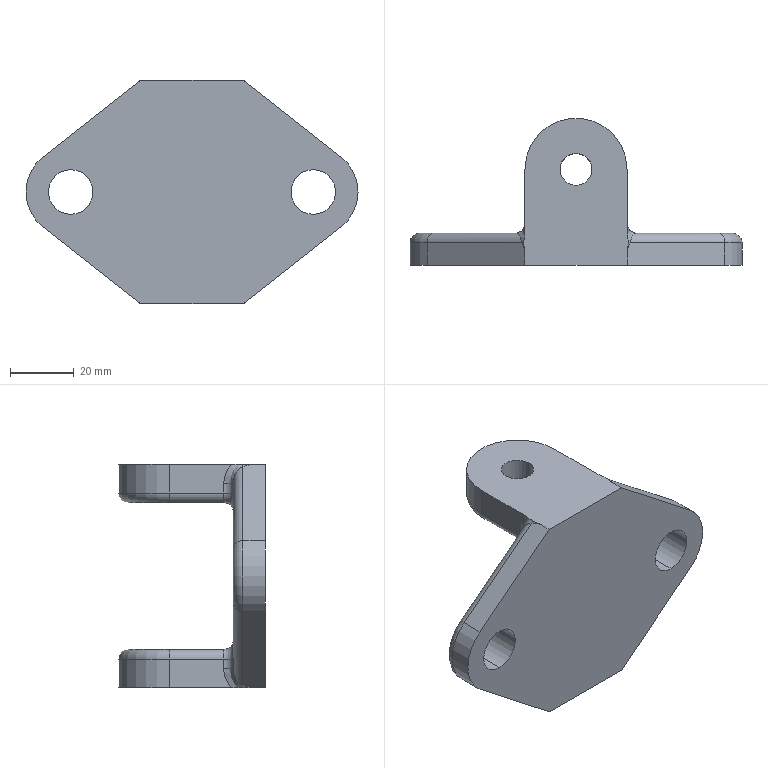Part | SolidWorks | features Fillet 3, Extrusion 1, ICE 1, MirrorPattern 1 | 1 solid | 54 faces | box 104 x 46 x 70 mm | volume 71759 mm3 | cylinder 26 | plane 14 | torus 8 | spline 6 | commonest cylinder face diameters 6 x14 10 x4 14 x4 28 x2 32 x2